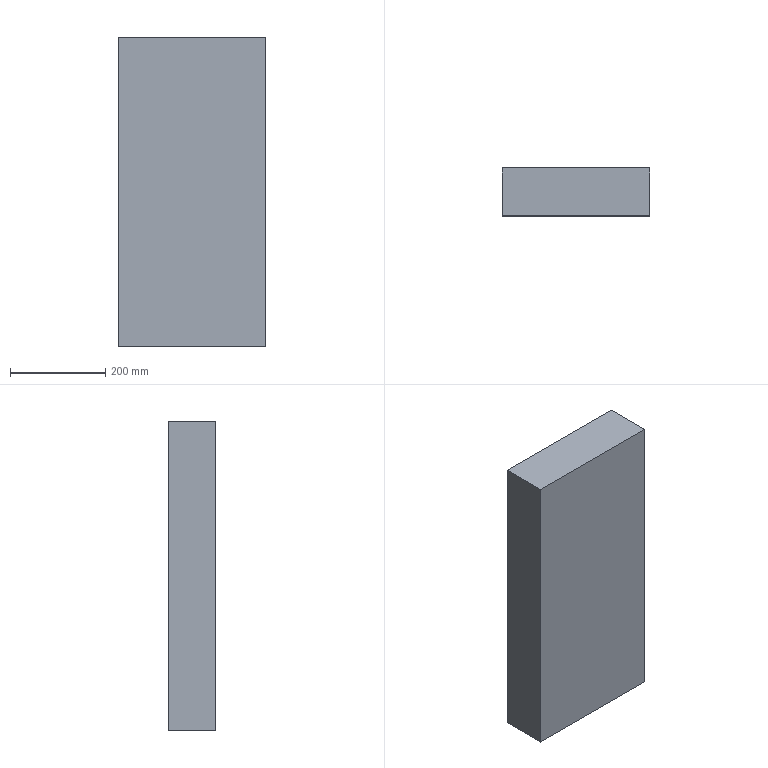Part | SolidWorks | features Extrusion 1 | 1 solid | 6 faces | box 310 x 100 x 650 mm | volume 20150000 mm3 | plane 6
STEP:
#1=CARTESIAN_POINT('',(155.,0.,325.));
#2=VERTEX_POINT('',#1);
#3=CARTESIAN_POINT('',(155.,0.,-325.));
#4=VERTEX_POINT('',#3);
#5=CARTESIAN_POINT('',(155.,0.,325.));
#6=DIRECTION('',(0.,0.,-1.));
#7=VECTOR('',#6,1000.);
#8=LINE('',#5,#7);
#9=EDGE_CURVE('',#2,#4,#8,.T.);
#10=ORIENTED_EDGE('',*,*,#9,.T.);
#11=CARTESIAN_POINT('',(155.,100.,-325.));
#12=VERTEX_POINT('',#11);
#13=CARTESIAN_POINT('',(155.,100.,-325.));
#14=DIRECTION('',(0.,-1.,0.));
#15=VECTOR('',#14,1000.);
#16=LINE('',#13,#15);
#17=EDGE_CURVE('',#12,#4,#16,.T.);
#18=ORIENTED_EDGE('',*,*,#17,.F.);
#19=CARTESIAN_POINT('',(155.,100.,325.));
#20=VERTEX_POINT('',#19);
#21=CARTESIAN_POINT('',(155.,100.,325.));
#22=DIRECTION('',(0.,0.,-1.));
#23=VECTOR('',#22,1000.);
#24=LINE('',#21,#23);
#25=EDGE_CURVE('',#20,#12,#24,.T.);
#26=ORIENTED_EDGE('',*,*,#25,.F.);
#27=CARTESIAN_POINT('',(155.,100.,325.));
#28=DIRECTION('',(0.,-1.,0.));
#29=VECTOR('',#28,1000.);
#30=LINE('',#27,#29);
#31=EDGE_CURVE('',#20,#2,#30,.T.);
#32=ORIENTED_EDGE('',*,*,#31,.T.);
#33=EDGE_LOOP('',(#10,#18,#26,#32));
#34=FACE_OUTER_BOUND('',#33,.T.);
#35=CARTESIAN_POINT('',(155.,100.,325.));
#36=DIRECTION('',(-1.,0.,0.));
#37=DIRECTION('',(0.,0.,1.));
#38=AXIS2_PLACEMENT_3D('',#35,#36,#37);
#39=PLANE('',#38);
#40=ADVANCED_FACE('',(#34),#39,.F.);
#41=CARTESIAN_POINT('',(-155.,0.,-325.));
#42=VERTEX_POINT('',#41);
#43=CARTESIAN_POINT('',(-155.,0.,-325.));
#44=DIRECTION('',(-1.,0.,0.));
#45=VECTOR('',#44,1000.);
#46=LINE('',#43,#45);
#47=EDGE_CURVE('',#4,#42,#46,.T.);
#48=ORIENTED_EDGE('',*,*,#47,.T.);
#49=CARTESIAN_POINT('',(-155.,100.,-325.));
#50=VERTEX_POINT('',#49);
#51=CARTESIAN_POINT('',(-155.,100.,-325.));
#52=DIRECTION('',(0.,-1.,0.));
#53=VECTOR('',#52,1000.);
#54=LINE('',#51,#53);
#55=EDGE_CURVE('',#50,#42,#54,.T.);
#56=ORIENTED_EDGE('',*,*,#55,.F.);
#57=CARTESIAN_POINT('',(-155.,100.,-325.));
#58=DIRECTION('',(-1.,0.,0.));
#59=VECTOR('',#58,1000.);
#60=LINE('',#57,#59);
#61=EDGE_CURVE('',#12,#50,#60,.T.);
#62=ORIENTED_EDGE('',*,*,#61,.F.);
#63=ORIENTED_EDGE('',*,*,#17,.T.);
#64=EDGE_LOOP('',(#48,#56,#62,#63));
#65=FACE_OUTER_BOUND('',#64,.T.);
#66=CARTESIAN_POINT('',(-155.,100.,-325.));
#67=DIRECTION('',(0.,0.,1.));
#68=DIRECTION('',(1.,0.,0.));
#69=AXIS2_PLACEMENT_3D('',#66,#67,#68);
#70=PLANE('',#69);
#71=ADVANCED_FACE('',(#65),#70,.F.);
#72=CARTESIAN_POINT('',(-155.,0.,325.));
#73=VERTEX_POINT('',#72);
#74=CARTESIAN_POINT('',(-155.,0.,325.));
#75=DIRECTION('',(0.,0.,1.));
#76=VECTOR('',#75,1000.);
#77=LINE('',#74,#76);
#78=EDGE_CURVE('',#42,#73,#77,.T.);
#79=ORIENTED_EDGE('',*,*,#78,.T.);
#80=CARTESIAN_POINT('',(-155.,100.,325.));
#81=VERTEX_POINT('',#80);
#82=CARTESIAN_POINT('',(-155.,100.,325.));
#83=DIRECTION('',(0.,-1.,0.));
#84=VECTOR('',#83,1000.);
#85=LINE('',#82,#84);
#86=EDGE_CURVE('',#81,#73,#85,.T.);
#87=ORIENTED_EDGE('',*,*,#86,.F.);
#88=CARTESIAN_POINT('',(-155.,100.,325.));
#89=DIRECTION('',(0.,0.,1.));
#90=VECTOR('',#89,1000.);
#91=LINE('',#88,#90);
#92=EDGE_CURVE('',#50,#81,#91,.T.);
#93=ORIENTED_EDGE('',*,*,#92,.F.);
#94=ORIENTED_EDGE('',*,*,#55,.T.);
#95=EDGE_LOOP('',(#79,#87,#93,#94));
#96=FACE_OUTER_BOUND('',#95,.T.);
#97=CARTESIAN_POINT('',(-155.,100.,325.));
#98=DIRECTION('',(1.,0.,0.));
#99=DIRECTION('',(0.,0.,-1.));
#100=AXIS2_PLACEMENT_3D('',#97,#98,#99);
#101=PLANE('',#100);
#102=ADVANCED_FACE('',(#96),#101,.F.);
#103=CARTESIAN_POINT('',(-155.,0.,325.));
#104=DIRECTION('',(1.,0.,0.));
#105=VECTOR('',#104,1000.);
#106=LINE('',#103,#105);
#107=EDGE_CURVE('',#73,#2,#106,.T.);
#108=ORIENTED_EDGE('',*,*,#107,.T.);
#109=ORIENTED_EDGE('',*,*,#31,.F.);
#110=CARTESIAN_POINT('',(-155.,100.,325.));
#111=DIRECTION('',(1.,0.,0.));
#112=VECTOR('',#111,1000.);
#113=LINE('',#110,#112);
#114=EDGE_CURVE('',#81,#20,#113,.T.);
#115=ORIENTED_EDGE('',*,*,#114,.F.);
#116=ORIENTED_EDGE('',*,*,#86,.T.);
#117=EDGE_LOOP('',(#108,#109,#115,#116));
#118=FACE_OUTER_BOUND('',#117,.T.);
#119=CARTESIAN_POINT('',(-155.,100.,325.));
#120=DIRECTION('',(0.,0.,-1.));
#121=DIRECTION('',(-1.,0.,0.));
#122=AXIS2_PLACEMENT_3D('',#119,#120,#121);
#123=PLANE('',#122);
#124=ADVANCED_FACE('',(#118),#123,.F.);
#125=ORIENTED_EDGE('',*,*,#25,.T.);
#126=ORIENTED_EDGE('',*,*,#61,.T.);
#127=ORIENTED_EDGE('',*,*,#92,.T.);
#128=ORIENTED_EDGE('',*,*,#114,.T.);
#129=EDGE_LOOP('',(#125,#126,#127,#128));
#130=FACE_OUTER_BOUND('',#129,.T.);
#131=CARTESIAN_POINT('',(0.,100.,0.));
#132=DIRECTION('',(0.,-1.,0.));
#133=DIRECTION('',(0.,0.,-1.));
#134=AXIS2_PLACEMENT_3D('',#131,#132,#133);
#135=PLANE('',#134);
#136=ADVANCED_FACE('',(#130),#135,.F.);
#137=ORIENTED_EDGE('',*,*,#9,.F.);
#138=ORIENTED_EDGE('',*,*,#107,.F.);
#139=ORIENTED_EDGE('',*,*,#78,.F.);
#140=ORIENTED_EDGE('',*,*,#47,.F.);
#141=EDGE_LOOP('',(#137,#138,#139,#140));
#142=FACE_OUTER_BOUND('',#141,.T.);
#143=CARTESIAN_POINT('',(0.,0.,0.));
#144=DIRECTION('',(0.,-1.,0.));
#145=DIRECTION('',(0.,0.,-1.));
#146=AXIS2_PLACEMENT_3D('',#143,#144,#145);
#147=PLANE('',#146);
#148=ADVANCED_FACE('',(#142),#147,.T.);
#149=CLOSED_SHELL('',(#40,#71,#102,#124,#136,#148));
#150=MANIFOLD_SOLID_BREP('',#149);
#151=CARTESIAN_POINT('',(0.,0.,0.));
#152=DIRECTION('',(0.,0.,1.));
#153=DIRECTION('',(1.,0.,0.));
#154=AXIS2_PLACEMENT_3D('',#151,#152,#153);
#155=(LENGTH_UNIT()NAMED_UNIT(*)SI_UNIT(.MILLI.,.METRE.));
#156=UNCERTAINTY_MEASURE_WITH_UNIT(LENGTH_MEASURE(0.00001),#155,'','');
#157=(NAMED_UNIT(*)PLANE_ANGLE_UNIT()SI_UNIT($,.RADIAN.));
#158=(NAMED_UNIT(*)SI_UNIT($,.STERADIAN.)SOLID_ANGLE_UNIT());
#159=(GEOMETRIC_REPRESENTATION_CONTEXT(3)GLOBAL_UNCERTAINTY_ASSIGNED_CONTEXT((#156))GLOBAL_UNIT_ASSIGNED_CONTEXT((#155,#157,#158))REPRESENTATION_CONTEXT('',''));
#160=ADVANCED_BREP_SHAPE_REPRESENTATION('',(#150,#154),#159);